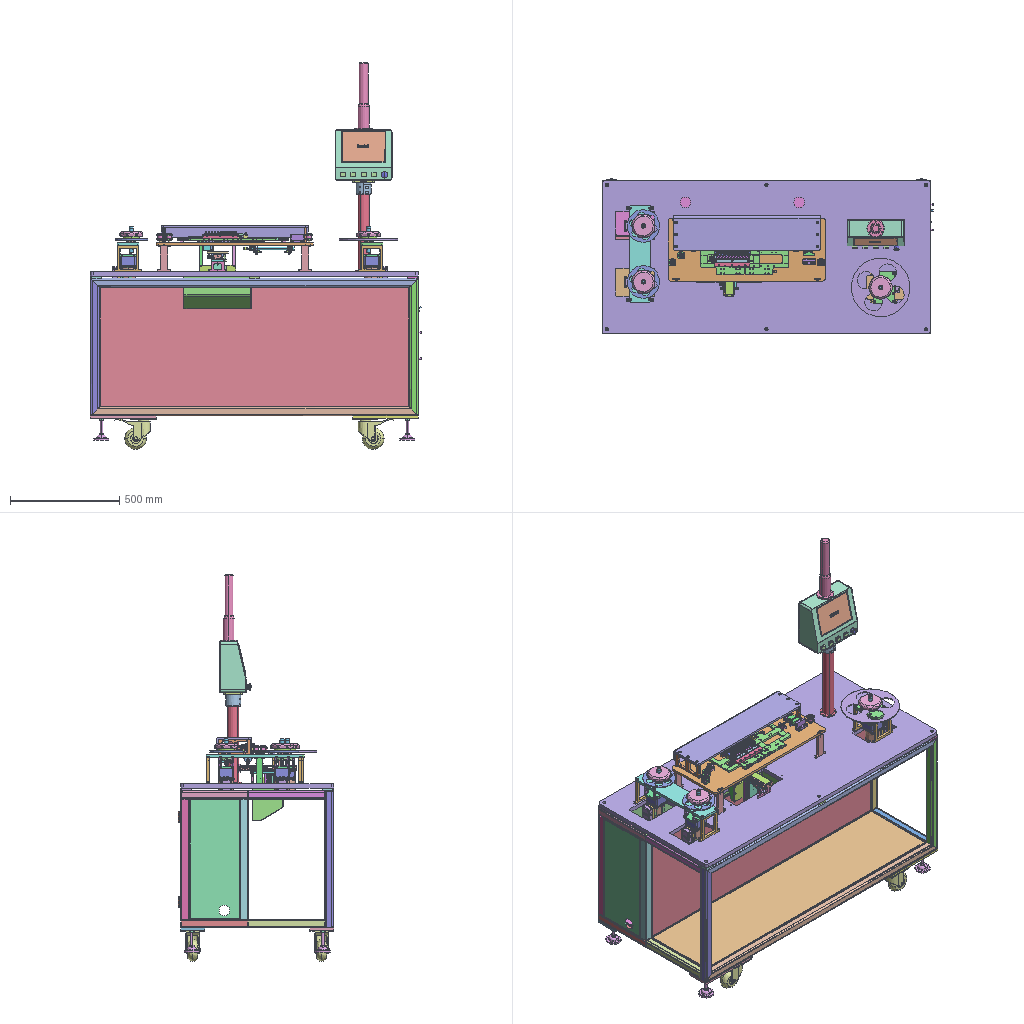Assembly | STEP file | 124 different items | 329 placed | box 1515 x 711 x 1768 mm
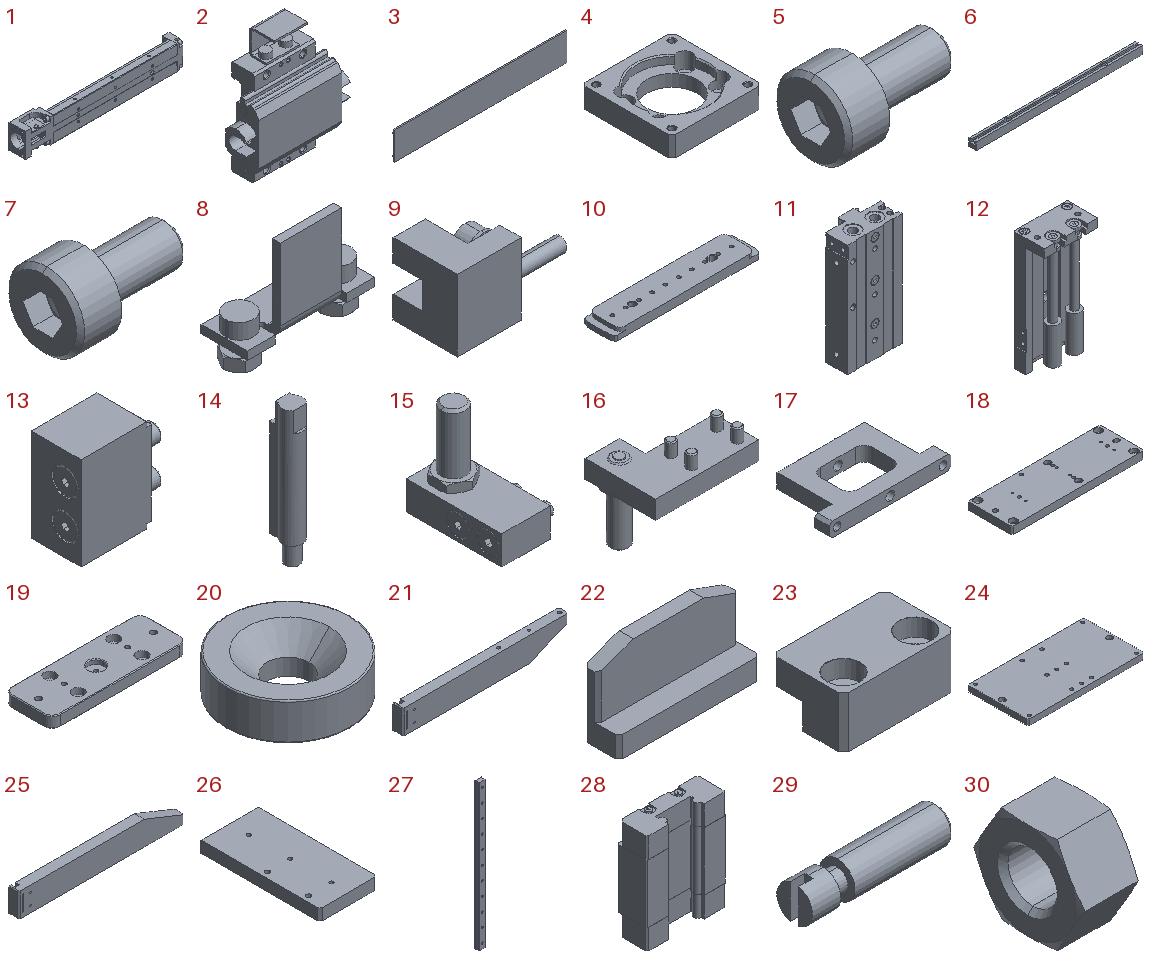Parts list (item | name | quantity | parent item | size | volume):
1 | QA-LX2005C_B1_A2038_200_EP3_b | x1 | in QA-LX2005C_B1_A2038_200_EP3 | 256 x 26.5 x 40 mm | 92553 mm3
2 | QA-LX2005C_B1_200_EP3_bl | x1 | in QA-LX2005C_B1_A2038_200_EP3 | 57 x 21 x 65.9 mm | 27894 mm3
3 | QA-LX2005C_B1_200_c | x1 | in QA-LX2005C_B1_A2038_200_EP3 | 216 x 3.2 x 35 mm | 15277 mm3
4 | QA-lx2001_A2038 | x1 | in QA-LX2005C_B1_A2038_200_EP3 | 38 x 38 x 8.5 mm | 7170 mm3
5 | QA-BOLT3_6 | x4 | in QA-LX2005C_B1_A2038_200_EP3 | 9 x 5.5 x 5.5 mm | 103.858 mm3
6 | QA-SENAT33H_208_V44_W104_X164_N3_5 | x1 | in QA-LX2005C_B1_A2038_200_EP3 | 208 x 9 x 9.5 mm | 12749 mm3
7 | QA-SCB3_6 | x3 | in QA-LX2005C_B1_A2038_200_EP3 | 9 x 5.5 x 5.5 mm | 103.858 mm3
8 | QA-PHOTO_SENSOR_br | x3 | in QA-LX2005C_B1_A2038_200_EP3 | 25.351 x 9 x 21 mm | 917.475 mm3
9 | QA-EE_SX91_R1M_lx | x3 | in QA-LX2005C_B1_A2038_200_EP3 | 21.25 x 12 x 14 mm | 1345 mm3
10 | QA-FB01 | x1 | in QA-FB0A | 150 x 32 x 9 mm | 39944 mm3
11 | QA-HI_MDX12x50-SD2BM2(0)_Bo | x1 | in QA-MDX12x50-SD2BM2 | 50 x 26.5 x 102 mm | 80346 mm3
12 | QA-HI_MDX12x50-SD2BM2(0)_Ro | x2 | in QA-MDX12x50-SD2BM2, QA-FB00 | 50 x 29 x 111 mm | 66088 mm3
13 | QA-HI_MDX-12 B | x1 | in QA-MDX12x50-SD2BM2 | 19.5 x 11 x 20.5 mm | 3566 mm3
14 | QA-HI_MDX-SD_2 | x2 | in QA-MDX12x50-SD2BM2 | 4 x 5.1 x 27.5 mm | 387.922 mm3
15 | QA-HI_MDX12_FB | x1 | in QA-MDX12x50-SD2BM2 | 20 x 31.5 x 33.5 mm | 6201 mm3
16 | QA-HI_MDX12_BB | x1 | in QA-MDX12x50-SD2BM2 | 45 x 31 x 38.5 mm | 10085 mm3
17 | QA-FB04 | x2 | in QA-FB00 | 84 x 48 x 10 mm | 20623 mm3
18 | QA-FB03 | x1 | in QA-FB00 | 180 x 60 x 10 mm | 103545 mm3
19 | QA-FB05 | x1 | in QA-FB00 | 96 x 34 x 8 mm | 24043 mm3
20 | QA-KZH10-3 | x1 | in QA-FB00 | 10 x 10 x 3 mm | 188.741 mm3
21 | QA-FB06 | x1 | in QA-FB00 | 206 x 12 x 30 mm | 66556 mm3
22 | QA-FB07 | x2 | in QA-FB00 | 20 x 5 x 11 mm | 541.763 mm3
23 | QA-FB08 | x2 | in QA-FB00 | 22 x 14 x 10 mm | 1976 mm3
24 | QA-FB09 | x1 | in QA-FB00 | 164 x 86 x 8 mm | 109937 mm3
25 | QA- Mirror FB06 | x1 | in QA-FB00 | 206 x 12 x 30 mm | 66556 mm3
26 | QA-FB10 | x1 | in QA-FB00 | 50 x 104 x 10 mm | 50937 mm3
27 | QA-r_SE2BL13_270 | x3 | in QA-SE2BL13_270, QA-SE2BL13_270-1, QA-0000-160616 | 12 x 7.5 x 270 mm | 21190 mm3
28 | QA-b_SEB13 | x6 | in QA-SE2BL13_270, QA-SE2BL13_270-1, QA-0000-160616 | 27 x 10 x 33.9 mm | 6982 mm3
29 | QA-BSPO5_20b | x11 | in QA-BSPO5_20, QA-BSPO5_20-1, QA-BSPO5_20-2, QA-BSPO5_20-3, QA-BSPO5_20-4, QA-BSPO5_20-5, QA-BSPO5_20-6, QA-BSPO5_20-7, QA-BSPO5_20-8, QA-BSPO5_20-9, QA-BSPO5_20-10 | 20 x 5 x 5 mm | 353.917 mm3
30 | QA-M5x0_8A | x22 | in QA-BSPO5_20, QA-BSPO5_25, QA-BSPO5_25-1, QA-BSPO5_25-2, QA-BSPO5_25-3, QA-BSPO5_25-4, QA-BSPO5_25-5, QA-BSPO5_25-6, QA-BSPO5_25-7, QA-BSPO5_25-8, QA-BSPO5_25-9, QA-BSPO5_25-10, QA-BSPO5_20-1, QA-BSPO5_20-2, QA-BSPO5_20-3, QA-BSPO5_20-4, QA-BSPO5_20-5, QA-BSPO5_20-6, QA-BSPO5_20-7, QA-BSPO5_20-8, QA-BSPO5_20-9, QA-BSPO5_20-10 | 4.7 x 9.238 x 8 mm | 194.282 mm3
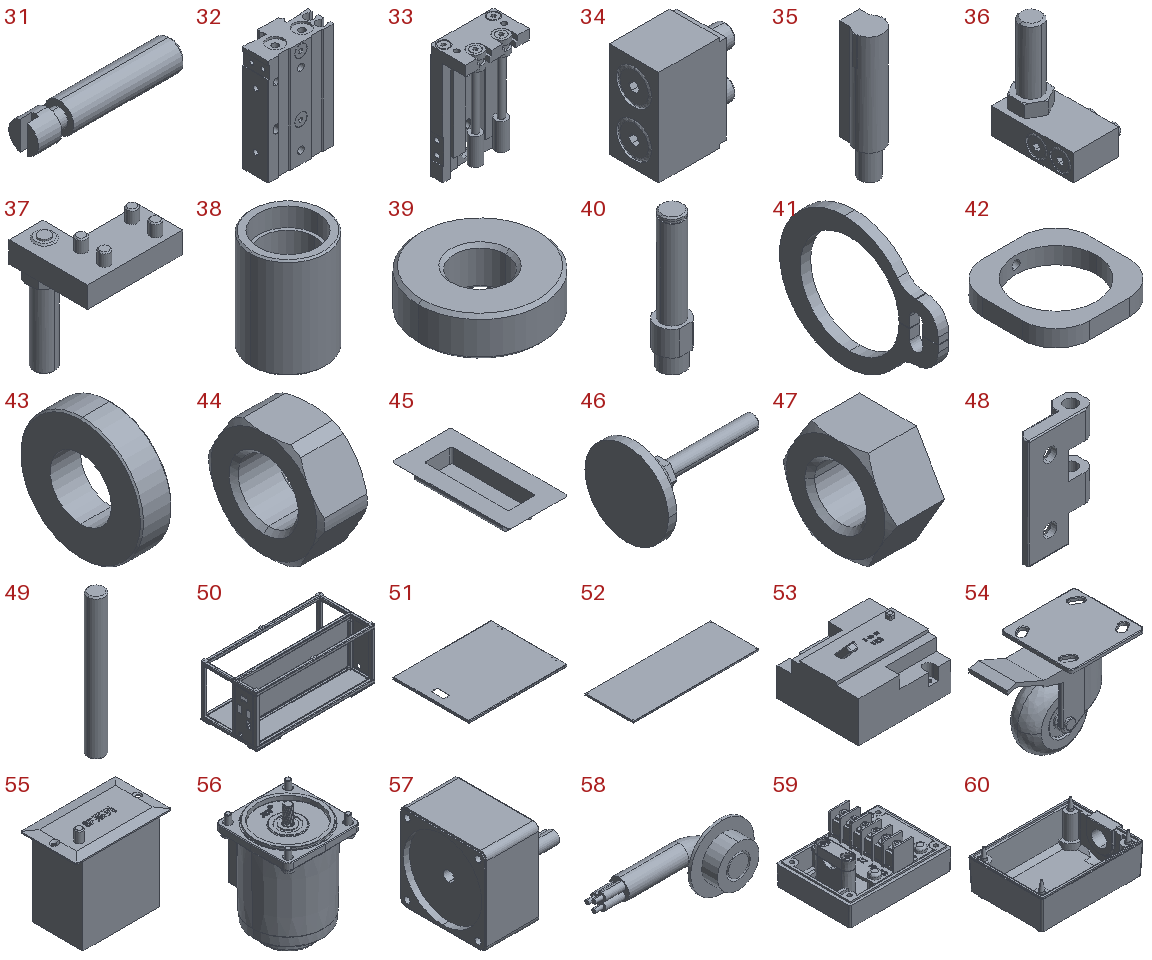31 | QA-BSPO5_25b | x11 | in QA-BSPO5_25, QA-BSPO5_25-1, QA-BSPO5_25-2, QA-BSPO5_25-3, QA-BSPO5_25-4, QA-BSPO5_25-5, QA-BSPO5_25-6, QA-BSPO5_25-7, QA-BSPO5_25-8, QA-BSPO5_25-9, QA-BSPO5_25-10 | 25 x 5 x 5 mm | 452.091 mm3
32 | QA-HI_MDX6x20-SG2BM2(0)_Bo | x1 | in QA-MDX6x20-SG2BM2 | 32 x 16 x 51.5 mm | 16782 mm3
33 | QA-HI_MDX6x20-SG2BM2(0)_Ro | x1 | in QA-MDX6x20-SG2BM2 | 32 x 18.5 x 57 mm | 12589 mm3
34 | QA-HI_MDX-6 B | x1 | in QA-MDX6x20-SG2BM2 | 13 x 7 x 13.5 mm | 935.094 mm3
35 | QA-HI_MDX-SG_2 | x2 | in QA-MDX6x20-SG2BM2 | 4 x 4.8 x 18 mm | 219.808 mm3
36 | QA-HI_MDX6_FB | x1 | in QA-MDX6x20-SG2BM2 | 13 x 19 x 26.37 mm | 1670 mm3
37 | QA-HI_MDX6_BB | x1 | in QA-MDX6x20-SG2BM2 | 22.5 x 18.7 x 29.3 mm | 2038 mm3
38 | QA-FC01 | x3 | in QA-FC00, QA-FC00-1, QA-FC00-2 | 24 x 24 x 32 mm | 6516 mm3
39 | QA-B698ZZ | x6 | in QA-FC00, QA-FC00-1, QA-FC00-2 | 19 x 19 x 6 mm | 1378 mm3
40 | QA-FC02 | x3 | in QA-FC00, QA-FC00-1, QA-FC00-2 | 11 x 10 x 49 mm | 2709 mm3
41 | QA-STWN8 | x3 | in QA-FC00, QA-FC00-1, QA-FC00-2 | 0.8 x 12.2 x 10 mm | 32.103 mm3
42 | QA-FC03 | x6 | in QA-FC00, QA-FC00-1, QA-FC00-2 | 32 x 32 x 5 mm | 2390 mm3
43 | QA-UWAUNS_washer-1 | x4 | in QA-UWAUNS-1, QA-UWAUNS-1-1 | 2 x 8 x 8 mm | 75.149 mm3
44 | QA-UWAUNS_nut-1 | x4 | in QA-UWAUNS-1, QA-UWAUNS-1-1 | 3.2 x 7.66 x 7 mm | 92.292 mm3
45 | QA-UWAUNS_1-1 | x2 | in QA-UWAUNS-1, QA-UWAUNS-1-1 | 60 x 120 x 15 mm | 28231 mm3
46 | QA-FJGN12_75pad-1 | x4 | in QA-FJGN12_75-1, QA-FJGN12_75-1-1, QA-FJGN12_75-1-2, QA-FJGN12_75-1-3 | 106 x 70 x 70 mm | 59651 mm3
47 | QA-FJGN12screw-1 | x4 | in QA-FJGN12_75-1, QA-FJGN12_75-1-1, QA-FJGN12_75-1-2, QA-FJGN12_75-1-3 | 10 x 21.939 x 19 mm | 2287 mm3
48 | QA-KHA50-1-1 | x8 | in QA-KHA50-1, 48, QA-KHA50-1-2, QA-KHA50-1-3 | 31 x 11.3 x 50 mm | 6837 mm3
49 | QA-KHA50-2-1 | x4 | in QA-KHA50-1, 48, QA-KHA50-1-2, QA-KHA50-1-3 | 6 x 6 x 50 mm | 1409 mm3
50 | QA-机箱-1(Default_As Machined_) | x1 | in QA-AD19 | 1500 x 700 x 650 mm | 12485783 mm3
51 | QA-Door panel B-1 | x2 | in QA-AD19 | 708 x 546 x 16.5 mm | 666860 mm3
52 | QA-衬Plate-1 | x1 | in QA-AD19 | 1416 x 546 x 18 mm | 1751680 mm3
53 | QA-N-33-HV-1 | x1 | in QA-AD19 | 90 x 80 x 56.121 mm | 279078 mm3
54 | QA-KVJHX100-1 | x4 | in QA-AD19 | 188.5 x 110 x 144.462 mm | 504709 mm3
55 | QA-SF系列调整器-1 | x3 | in QA-AD19 | 102 x 60 x 101 mm | 397007 mm3
56 | QA-15YT01-25-1 | x3 | in QA-15YT01-25, 56, 57 | 71.679 x 71.19 x 107.5 mm | 89869 mm3
57 | QA-15YT01-25-2 | x3 | in QA-15YT01-25, 56, 57 | 76 x 70.5 x 70.5 mm | 194650 mm3
58 | QA-15YT01-25-3 | x3 | in QA-15YT01-25, 56, 57 | 35 x 12.5 x 16 mm | 1115 mm3
59 | QA-15YT01-25-4 | x3 | in QA-15YT01-25, 56, 57 | 67 x 49 x 34.5 mm | 31444 mm3
60 | QA-15YT01-25-5 | x3 | in QA-15YT01-25, 56, 57 | 73.93 x 48.93 x 29.5 mm | 22748 mm3
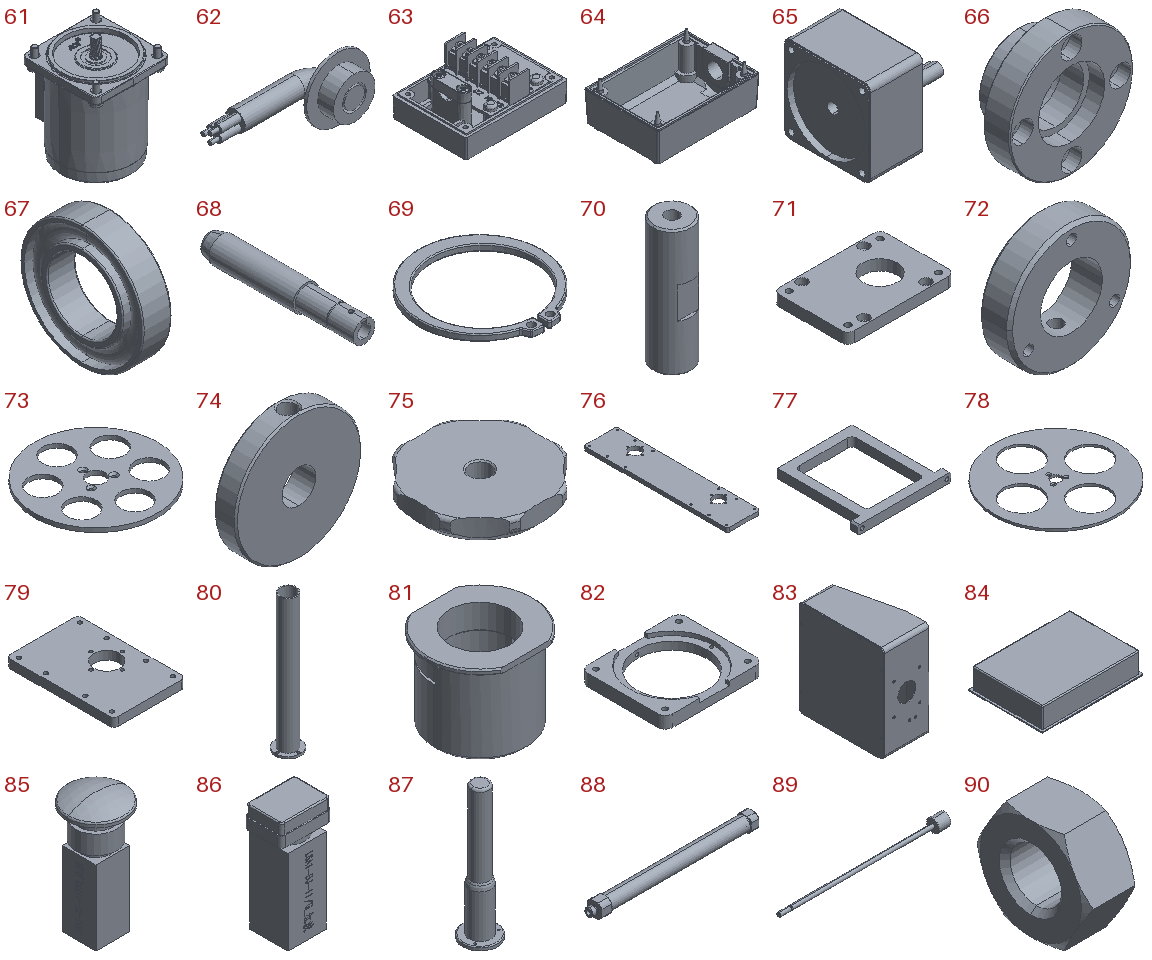61 | QA-70YS15G | x2 | in QA-06tp01-180, QA-06tp01-180-1 | 71.679 x 71.19 x 97.5 mm | 85810 mm3
62 | QA-YX_1 | x2 | in QA-06tp01-180, QA-06tp01-180-1 | 35 x 12.5 x 16 mm | 1115 mm3
63 | QA-JXH-X_1 | x2 | in QA-06tp01-180, QA-06tp01-180-1 | 67 x 49 x 34.5 mm | 31444 mm3
64 | QA-JXH-S_1 | x2 | in QA-06tp01-180, QA-06tp01-180-1 | 73.93 x 48.93 x 29.5 mm | 22748 mm3
65 | QA-70GK-H-180 | x2 | in QA-06tp01-180, QA-06tp01-180-1 | 76 x 70.5 x 70.5 mm | 194650 mm3
66 | QA-FC10 | x3 | in QA-Material discharge module, QA-放料模组-1, QA-Material receiving module | 56 x 24 x 56 mm | 24731 mm3
67 | QA-Bearing-B6903ZZ | x6 | in QA-Material discharge module, QA-放料模组-1, QA-Material receiving module | 7 x 30 x 30 mm | 2496 mm3
68 | QA-FC09 | x3 | in QA-Material discharge module, QA-放料模组-1, QA-Material receiving module | 20 x 120 x 19.5 mm | 30201 mm3
69 | QA-Retaining ring-KSTW17 | x3 | in QA-Material discharge module, QA-放料模组-1, QA-Material receiving module | 18.84 x 19.765 x 1 mm | 85.594 mm3
70 | QA-FC07 | x12 | in QA-Material discharge module, QA-放料模组-1, QA-Material receiving module | 12 x 12 x 40 mm | 4081 mm3
71 | QA-FC08 | x3 | in QA-Material discharge module, QA-放料模组-1, QA-Material receiving module | 100 x 70 x 10 mm | 57674 mm3
72 | QA-FC11 | x3 | in QA-Material discharge module, QA-放料模组-1, QA-Material receiving module | 40 x 10 x 40 mm | 8899 mm3
73 | QA-FC12 | x2 | in QA-Material discharge module, QA-放料模组-1 | 150 x 150 x 5 mm | 57214 mm3
74 | QA-FC15 | x3 | in QA-Material discharge module, QA-放料模组-1, QA-Material receiving module | 75 x 13 x 74.963 mm | 51433 mm3
75 | QA-FC13 | x3 | in QA-Material discharge module, QA-放料模组-1, QA-Material receiving module | 104.038 x 104.038 x 20 mm | 157045 mm3
76 | QA-FC04 | x1 | in QA-FC0A | 100 x 440 x 12 mm | 495046 mm3
77 | QA-FC06 | x4 | in QA-FC0A, QA-FC0B | 124 x 120 x 12 mm | 58795 mm3
78 | QA-FC14 | x1 | in QA-Material receiving module | 270 x 270 x 5 mm | 183467 mm3
79 | QA-FC05 | x1 | in QA-FC0B | 100 x 150 x 12 mm | 162249 mm3
80 | QA-TE01 | x1 | in QA-TE00 | 74 x 74 x 400 mm | 190414 mm3
81 | QA-TE02 | x1 | in QA-TE00 | 80 x 70 x 64 mm | 121771 mm3
82 | QA-TE03 | x1 | in QA-TE00 | 100 x 86 x 12 mm | 46511 mm3
83 | QA-TE04 | x1 | in QA-TE00 | 123 x 230 x 260 mm | 391275 mm3
84 | QA-MT6070IH | x1 | in QA-TE00 | 200 x 146 x 43 mm | 1146130 mm3
85 | QA-LSA1-BY-11TSB | x1 | in QA-TE00 | 30.8 x 30.8 x 65 mm | 21898 mm3
86 | QA-LSA1-BJ-11 | x4 | in QA-TE00 | 24 x 18 x 53 mm | 17646 mm3
87 | QA-TPWB4-L73ROG | x1 | in QA-TE00 | 80 x 80 x 307 mm | 491038 mm3
88 | QA-HI_SBA16x150-SB2-LB_B | x1 | in QA-SBA16x150-SB2-LB | 205 x 18 x 18 mm | 13813 mm3
89 | QA-HI_SBA16x150-LB_R | x1 | in QA-SBA16x150-SB2-LB | 210.5 x 16 x 16 mm | 6843 mm3
90 | QA-HI_N-M5x0.8_3 | x1 | in QA-SBA16x150-SB2-LB | 4 x 9.238 x 8 mm | 164.283 mm3
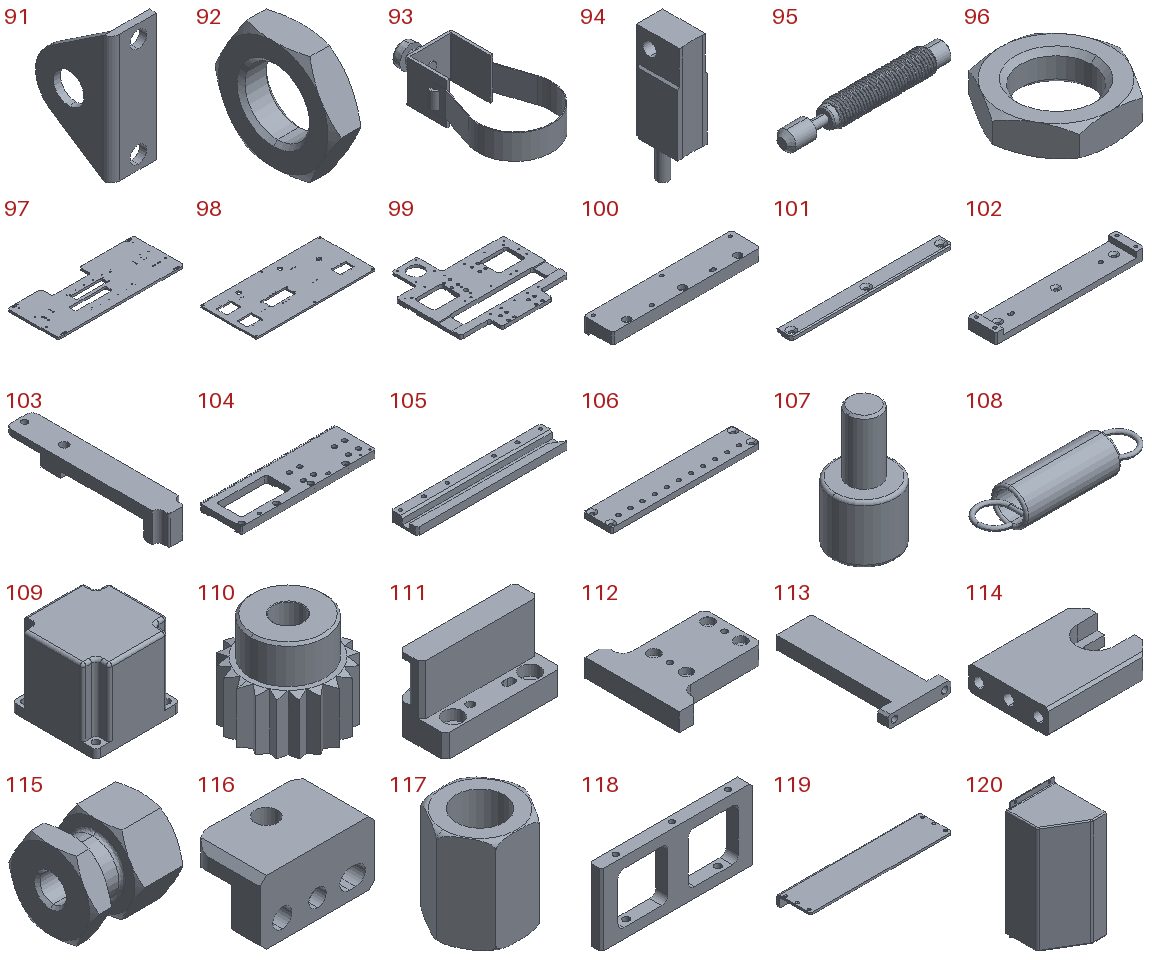91 | QA-HI_SBA-16-LB_(150) | x1 | in QA-SBA16x150-SB2-LB | 15 x 25 x 42 mm | 2467 mm3
92 | QA-HI_N-M10x1.0_3 | x1 | in QA-SBA16x150-SB2-LB | 4 x 17.321 x 15 mm | 513.744 mm3
93 | QA-HI_SBA16-SM_3 | x2 | in QA-SBA16x150-SB2-LB | 17.8 x 35.9 x 10 mm | 369.6 mm3
94 | QA-HI_SB-CS-130_3 | x2 | in QA-SBA16x150-SB2-LB | 8 x 11.8 x 36 mm | 2270 mm3
95 | QA-SKSC0806-1 | x2 | in QA-SKSC0806, 95 | 55.353 x 8 x 8 mm | 1947 mm3
96 | QA-SKSC0806-2 | x4 | in QA-SKSC0806, 95 | 12.702 x 11 x 3 mm | 190.264 mm3
97 | QA-AD01 | x1 | in QA-0000-160616 | 720 x 288 x 12 mm | 2124409 mm3
98 | QA-AD02 | x1 | in QA-0000-160616 | 1500 x 700 x 20 mm | 18757856 mm3
99 | QA-AD03 | x2 | in QA-0000-160616 | 270 x 258 x 10 mm | 320540 mm3
100 | QA-AD04 | x1 | in QA-0000-160616 | 160 x 32 x 15.1 mm | 62990 mm3
101 | QA-AD05 | x1 | in QA-0000-160616 | 160 x 16 x 4 mm | 9462 mm3
102 | QA-AD06 | x1 | in QA-0000-160616 | 166.5 x 32 x 12 mm | 34292 mm3
103 | QA-AD07 | x11 | in QA-0000-160616 | 13.5 x 80 x 14.8 mm | 6677 mm3
104 | QA-AD08 | x1 | in QA-0000-160616 | 195 x 60 x 10 mm | 78945 mm3
105 | QA-AD09 | x1 | in QA-0000-160616 | 160 x 28 x 10.5 mm | 32238 mm3
106 | QA-AD10 | x1 | in QA-0000-160616 | 166.5 x 32 x 6 mm | 30437 mm3
107 | QA-CFM3-6 | x11 | in QA-0000-160616 | 6 x 6 x 11.5 mm | 192.07 mm3
108 | QA-AWU6_25 | x11 | in QA-0000-160616 | 26.4 x 6 x 6 mm | 193.836 mm3
109 | QA-SM57-51C | x1 | in QA-0000-160616 | 56.4 x 56.4 x 73.2 mm | 150583 mm3
110 | QA-GER1.0-20-W12-B-H6.35 | x1 | in QA-0000-160616 | 22 x 22 x 20 mm | 4666 mm3
111 | QA-AD11 | x1 | in QA-0000-160616 | 60 x 24 x 38 mm | 30322 mm3
112 | QA-AD12 | x1 | in QA-0000-160616 | 56 x 52 x 10 mm | 19264 mm3
113 | QA-AD13 | x4 | in QA-0000-160616 | 60 x 120 x 12 mm | 50441 mm3
114 | QA-AD14 | x1 | in QA-0000-160616 | 43 x 32 x 10 mm | 11347 mm3
115 | QA-KFJR5-0.8-4 | x1 | in QA-0000-160616 | 14 x 13.856 x 12 mm | 1253 mm3
116 | QA-AD15 | x2 | in QA-0000-160616 | 36 x 22 x 20 mm | 8518 mm3
117 | QA-SKST801 | x2 | in QA-0000-160616 | 12.702 x 11 x 14 mm | 925.966 mm3
118 | QA-AD17 | x2 | in QA-0000-160616 | 150 x 12 x 70 mm | 65829 mm3
119 | QA-AD16 | x1 | in QA-0000-160616 | 672 x 160 x 55 mm | 1359289 mm3
120 | QA-AD18 | x1 | in QA-0000-160616 | 140 x 150 x 342 mm | 227668 mm3
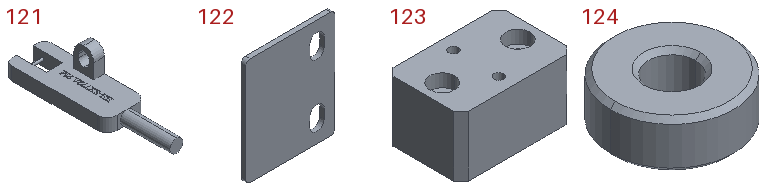121 | QA-EE-SX772A 2M | x1 | in QA-0000-160616 | 12 x 46 x 19.1 mm | 1673 mm3
122 | QA-AD20 | x1 | in QA-0000-160616 | 20 x 1 x 24 mm | 450.257 mm3
123 | QA-AD21 | x1 | in QA-0000-160616 | 30 x 20 x 16 mm | 8932 mm3
124 | QA-KGHA5-13 | x3 | in QA-0000-160616 | 13 x 13 x 5 mm | 551.35 mm3
Placements (level | parent | child | x y z in mm | rotation matrix by rows), first 242 of 386 lines:
1 | QA-0000-160616 | QA-FB00 | -62.867 62.015 497.223 | 1 0 0 0 0 -1 0 1 0
2 | QA-FB00 | QA-LX2005C_B1_A2038_200_EP3 | -1.553 34.777 194.0 | 0 0 -1 0 1 0 1 0 0
3 | QA-LX2005C_B1_A2038_200_EP3 | QA-LX2005C_B1_A2038_200_EP3_b | -128.0 -0.0 -0.0 | 1 0 0 0 1 0 0 0 1
3 | QA-LX2005C_B1_A2038_200_EP3 | QA-LX2005C_B1_200_EP3_bl | -42.0 -0.0 -0.0 | 1 0 0 0 1 0 0 0 1
3 | QA-LX2005C_B1_A2038_200_EP3 | QA-LX2005C_B1_200_c | -128.0 -0.0 -0.0 | 1 0 0 0 1 0 0 0 1
3 | QA-LX2005C_B1_A2038_200_EP3 | QA-lx2001_A2038 | -132.25 13.0 -0.0 | 0 0 -1 0 1 0 1 0 0
3 | QA-LX2005C_B1_A2038_200_EP3 | QA-BOLT3_6 | -129.8 5.75 -12.557 | 1 0 0 0 -1 0 0 0 -1
3 | QA-LX2005C_B1_A2038_200_EP3 | QA-BOLT3_6 | -129.8 20.25 12.557 | 1 0 0 0 -1 0 0 0 -1
3 | QA-LX2005C_B1_A2038_200_EP3 | QA-BOLT3_6 | -129.8 20.25 -12.557 | 1 0 0 0 -1 0 0 0 -1
3 | QA-LX2005C_B1_A2038_200_EP3 | QA-BOLT3_6 | -129.8 5.75 12.557 | 1 0 0 0 -1 0 0 0 -1
3 | QA-LX2005C_B1_A2038_200_EP3 | QA-SENAT33H_208_V44_W104_X164_N3_5 | -86.0 5.5 20.0 | 1 0 0 0 1 0 0 0 1
3 | QA-LX2005C_B1_A2038_200_EP3 | QA-SCB3_6 | 78.0 5.5 22.0 | 0 0 -1 0 -1 0 -1 0 0
3 | QA-LX2005C_B1_A2038_200_EP3 | QA-SCB3_6 | -42.0 5.5 22.0 | 0 0 -1 0 -1 0 -1 0 0
3 | QA-LX2005C_B1_A2038_200_EP3 | QA-SCB3_6 | 18.0 5.5 22.0 | 0 0 -1 0 -1 0 -1 0 0
3 | QA-LX2005C_B1_A2038_200_EP3 | QA-PHOTO_SENSOR_br | -38.0 1.0 29.5 | 1 0 0 0 1 0 0 0 1
3 | QA-LX2005C_B1_A2038_200_EP3 | QA-PHOTO_SENSOR_br | 74.0 1.0 29.5 | 1 0 0 0 1 0 0 0 1
3 | QA-LX2005C_B1_A2038_200_EP3 | QA-PHOTO_SENSOR_br | 18.0 1.0 29.5 | 1 0 0 0 1 0 0 0 1
3 | QA-LX2005C_B1_A2038_200_EP3 | QA-EE_SX91_R1M_lx | 74.0 2.6 46.1 | -1 0 0 0 1 0 0 0 -1
3 | QA-LX2005C_B1_A2038_200_EP3 | QA-EE_SX91_R1M_lx | -38.0 2.6 46.1 | -1 0 0 0 1 0 0 0 -1
3 | QA-LX2005C_B1_A2038_200_EP3 | QA-EE_SX91_R1M_lx | 18.0 2.6 46.1 | -1 0 0 0 1 0 0 0 -1
2 | QA-FB00 | QA-FB0A | 1.597 -18.223 137.473 | 1 0 0 0 0 1 0 -1 0
3 | QA-FB0A | QA-FB01 | -3.15 -14.527 136.0 | 1 0 0 0 1 0 0 0 1
2 | QA-FB00 | QA-MDX12x50-SD2BM2 | -1.553 -79.223 207.0 | -1 0 0 0 0 -1 0 -1 0
3 | QA-MDX12x50-SD2BM2 | QA-HI_MDX12x50-SD2BM2(0)_Bo | -0.0 -0.0 -0.0 | 1 0 0 0 1 0 0 0 1
3 | QA-MDX12x50-SD2BM2 | QA-HI_MDX12x50-SD2BM2(0)_Ro | -0.0 -0.0 -0.0 | 1 0 0 0 1 0 0 0 1
3 | QA-MDX12x50-SD2BM2 | QA-HI_MDX-12 B | -25.0 24.0 -73.75 | 1 0 0 0 1 0 0 0 1
3 | QA-MDX12x50-SD2BM2 | QA-HI_MDX-SD_2 | 20.0 6.0 -102.0 | 0 1 0 1 0 0 0 0 -1
3 | QA-MDX12x50-SD2BM2 | QA-HI_MDX-SD_2 | 20.0 14.0 -0.0 | 0 1 0 -1 0 0 0 0 1
3 | QA-MDX12x50-SD2BM2 | QA-HI_MDX12_FB | -25.0 5.0 -6.75 | 1 0 0 0 1 0 0 0 1
3 | QA-MDX12x50-SD2BM2 | QA-HI_MDX12_BB | -0.0 5.0 -102.0 | 1 0 0 0 1 0 0 0 1
2 | QA-FB00 | QA-FB04 | -1.553 0.7766 115.0 | 1 0 0 0 1 0 0 0 1
2 | QA-FB00 | QA-FB04 | -1.553 0.7766 279.0 | 1 0 0 0 1 0 0 0 1
2 | QA-FB00 | QA-FB03 | -1.553 24.777 202.0 | 0 1 0 0 0 1 1 0 0
2 | QA-FB00 | QA-FB05 | -1.553 61.777 152.0 | 1 0 0 0 0 1 0 -1 0
2 | QA-FB00 | QA-KZH10-3 | -1.553 66.577 152.0 | 1 0 0 0 0 1 0 -1 0
2 | QA-FB00 | QA-FB06 | -83.553 125.877 137.0 | 0 1 0 -1 0 0 0 0 1
2 | QA-FB00 | QA-FB07 | 84.447 121.277 152.0 | 0 0 -1 0 1 0 1 0 -0
2 | QA-FB00 | QA-FB07 | -87.553 121.277 152.0 | 0 0 1 0 1 0 -1 0 -0
2 | QA-FB00 | QA-FB08 | 80.447 107.277 152.0 | 0 0 1 0 1 0 -1 0 0
2 | QA-FB00 | QA-FB08 | -83.553 107.277 152.0 | 0 0 -1 0 1 0 1 0 0
2 | QA-FB00 | QA-FB09 | -1.553 -37.123 167.0 | 1 0 0 0 1 0 0 0 1
2 | QA-FB00 | QA- Mirror FB06 | 80.447 125.877 137.0 | 0 -1 0 -1 0 0 0 0 -1
2 | QA-FB00 | QA-FB10 | -1.553 -27.223 217.0 | -1 0 0 0 1 0 0 0 -1
2 | QA-FB00 | QA-HI_MDX12x50-SD2BM2(0)_Ro | -1.553 -129.223 207.0 | -1 0 0 0 0 -1 0 -1 0
1 | QA-0000-160616 | QA-SE2BL13_270 | 148.58 -3.985 606.0 | 0 0 -1 -1 0 0 0 1 0
2 | QA-SE2BL13_270 | QA-r_SE2BL13_270 | -0.0 -0.0 -0.0 | 1 0 0 0 1 0 0 0 1
2 | QA-SE2BL13_270 | QA-b_SEB13 | -0.0 3.0 174.889 | 1 0 0 0 1 0 0 0 1
2 | QA-SE2BL13_270 | QA-b_SEB13 | -0.0 3.0 244.889 | 1 0 0 0 1 0 0 0 1
1 | QA-0000-160616 | QA-SE2BL13_270-1 | 148.58 -145.985 606.0 | 0 0 -1 -1 0 0 0 1 0
2 | QA-SE2BL13_270-1 | QA-r_SE2BL13_270 | -0.0 -0.0 -0.0 | 1 0 0 0 1 0 0 0 1
2 | QA-SE2BL13_270-1 | QA-b_SEB13 | -0.0 3.0 244.889 | 1 0 0 0 1 0 0 0 1
2 | QA-SE2BL13_270-1 | QA-b_SEB13 | -0.0 3.0 174.889 | 1 0 0 0 1 0 0 0 1
1 | QA-0000-160616 | QA-BSPO5_20 | -117.77 -65.985 660.0 | 0 -0.866 0.5 0 0.5 0.866 -1 0 -0
2 | QA-BSPO5_20 | QA-BSPO5_20b | -0.0 -0.0 -0.0 | 1 0 0 0 1 0 0 0 1
2 | QA-BSPO5_20 | QA-M5x0_8A | 12.65 0.0 -0.0 | -1 0 0 0 -1 0 0 0 1
1 | QA-0000-160616 | QA-BSPO5_25 | -118.42 -28.985 657.9 | 0 0 1 0 1 0 -1 0 0
2 | QA-BSPO5_25 | QA-M5x0_8A | 16.65 -0.0 -0.0 | -1 0 0 0 -1 0 0 0 1
2 | QA-BSPO5_25 | QA-BSPO5_25b | -0.0 -0.0 -0.0 | 1 0 0 0 1 0 0 0 1
1 | QA-0000-160616 | QA-BSPO5_25-1 | -104.92 -28.985 657.9 | 0 0 1 0 1 0 -1 0 0
2 | QA-BSPO5_25-1 | QA-M5x0_8A | 16.65 -0.0 -0.0 | -1 0 0 0 -1 0 0 0 1
2 | QA-BSPO5_25-1 | QA-BSPO5_25b | -0.0 -0.0 -0.0 | 1 0 0 0 1 0 0 0 1
1 | QA-0000-160616 | QA-BSPO5_25-2 | -91.42 -28.985 657.9 | 0 0 1 0 1 0 -1 0 0
2 | QA-BSPO5_25-2 | QA-M5x0_8A | 16.65 -0.0 -0.0 | -1 0 0 0 -1 0 0 0 1
2 | QA-BSPO5_25-2 | QA-BSPO5_25b | -0.0 -0.0 -0.0 | 1 0 0 0 1 0 0 0 1
1 | QA-0000-160616 | QA-BSPO5_25-3 | -77.92 -28.985 657.9 | 0 0 1 0 1 0 -1 0 0
2 | QA-BSPO5_25-3 | QA-M5x0_8A | 16.65 -0.0 -0.0 | -1 0 0 0 -1 0 0 0 1
2 | QA-BSPO5_25-3 | QA-BSPO5_25b | -0.0 -0.0 -0.0 | 1 0 0 0 1 0 0 0 1
1 | QA-0000-160616 | QA-BSPO5_25-4 | -64.42 -28.985 657.9 | 0 0 1 0 1 0 -1 0 0
2 | QA-BSPO5_25-4 | QA-M5x0_8A | 16.65 -0.0 -0.0 | -1 0 0 0 -1 0 0 0 1
2 | QA-BSPO5_25-4 | QA-BSPO5_25b | -0.0 -0.0 -0.0 | 1 0 0 0 1 0 0 0 1
1 | QA-0000-160616 | QA-BSPO5_25-5 | -50.92 -28.985 657.9 | 0 0 1 0 1 0 -1 0 0
2 | QA-BSPO5_25-5 | QA-M5x0_8A | 16.65 -0.0 -0.0 | -1 0 0 0 -1 0 0 0 1
2 | QA-BSPO5_25-5 | QA-BSPO5_25b | -0.0 -0.0 -0.0 | 1 0 0 0 1 0 0 0 1
1 | QA-0000-160616 | QA-BSPO5_25-6 | -37.42 -28.985 657.9 | 0 0 1 0 1 0 -1 0 0
2 | QA-BSPO5_25-6 | QA-M5x0_8A | 16.65 -0.0 -0.0 | -1 0 0 0 -1 0 0 0 1
2 | QA-BSPO5_25-6 | QA-BSPO5_25b | -0.0 -0.0 -0.0 | 1 0 0 0 1 0 0 0 1
1 | QA-0000-160616 | QA-BSPO5_25-7 | -23.92 -28.985 657.9 | 0 0 1 0 1 0 -1 0 0
2 | QA-BSPO5_25-7 | QA-M5x0_8A | 16.65 -0.0 -0.0 | -1 0 0 0 -1 0 0 0 1
2 | QA-BSPO5_25-7 | QA-BSPO5_25b | -0.0 -0.0 -0.0 | 1 0 0 0 1 0 0 0 1
1 | QA-0000-160616 | QA-BSPO5_25-8 | -10.42 -28.985 657.9 | 0 0 1 0 1 0 -1 0 0
2 | QA-BSPO5_25-8 | QA-M5x0_8A | 16.65 -0.0 -0.0 | -1 0 0 0 -1 0 0 0 1
2 | QA-BSPO5_25-8 | QA-BSPO5_25b | -0.0 -0.0 -0.0 | 1 0 0 0 1 0 0 0 1
1 | QA-0000-160616 | QA-BSPO5_25-9 | 3.08 -28.985 657.9 | 0 0 1 0 1 0 -1 0 0
2 | QA-BSPO5_25-9 | QA-M5x0_8A | 16.65 -0.0 -0.0 | -1 0 0 0 -1 0 0 0 1
2 | QA-BSPO5_25-9 | QA-BSPO5_25b | -0.0 -0.0 -0.0 | 1 0 0 0 1 0 0 0 1
1 | QA-0000-160616 | QA-BSPO5_25-10 | 16.58 -28.985 657.9 | 0 0 1 0 1 0 -1 0 0
2 | QA-BSPO5_25-10 | QA-M5x0_8A | 16.65 -0.0 -0.0 | -1 0 0 0 -1 0 0 0 1
2 | QA-BSPO5_25-10 | QA-BSPO5_25b | -0.0 -0.0 -0.0 | 1 0 0 0 1 0 0 0 1
1 | QA-0000-160616 | QA-BSPO5_20-1 | -104.27 -65.985 660.0 | 0 -0.866 0.5 0 0.5 0.866 -1 0 -0
2 | QA-BSPO5_20-1 | QA-BSPO5_20b | -0.0 -0.0 -0.0 | 1 0 0 0 1 0 0 0 1
2 | QA-BSPO5_20-1 | QA-M5x0_8A | 12.65 0.0 -0.0 | -1 0 0 0 -1 0 0 0 1
1 | QA-0000-160616 | QA-BSPO5_20-2 | -90.77 -65.985 660.0 | 0 -0.866 0.5 0 0.5 0.866 -1 0 -0
2 | QA-BSPO5_20-2 | QA-BSPO5_20b | -0.0 -0.0 -0.0 | 1 0 0 0 1 0 0 0 1
2 | QA-BSPO5_20-2 | QA-M5x0_8A | 12.65 0.0 -0.0 | -1 0 0 0 -1 0 0 0 1
1 | QA-0000-160616 | QA-BSPO5_20-3 | -77.27 -65.985 660.0 | 0 -0.866 0.5 0 0.5 0.866 -1 0 -0
2 | QA-BSPO5_20-3 | QA-BSPO5_20b | -0.0 -0.0 -0.0 | 1 0 0 0 1 0 0 0 1
2 | QA-BSPO5_20-3 | QA-M5x0_8A | 12.65 0.0 -0.0 | -1 0 0 0 -1 0 0 0 1
1 | QA-0000-160616 | QA-BSPO5_20-4 | -63.77 -65.985 660.0 | 0 -0.866 0.5 0 0.5 0.866 -1 0 -0
2 | QA-BSPO5_20-4 | QA-BSPO5_20b | -0.0 -0.0 -0.0 | 1 0 0 0 1 0 0 0 1
2 | QA-BSPO5_20-4 | QA-M5x0_8A | 12.65 0.0 -0.0 | -1 0 0 0 -1 0 0 0 1
1 | QA-0000-160616 | QA-BSPO5_20-5 | -50.27 -65.985 660.0 | 0 -0.866 0.5 0 0.5 0.866 -1 0 -0
2 | QA-BSPO5_20-5 | QA-BSPO5_20b | -0.0 -0.0 -0.0 | 1 0 0 0 1 0 0 0 1
2 | QA-BSPO5_20-5 | QA-M5x0_8A | 12.65 0.0 -0.0 | -1 0 0 0 -1 0 0 0 1
1 | QA-0000-160616 | QA-BSPO5_20-6 | -36.77 -65.985 660.0 | 0 -0.866 0.5 0 0.5 0.866 -1 0 -0
2 | QA-BSPO5_20-6 | QA-BSPO5_20b | -0.0 -0.0 -0.0 | 1 0 0 0 1 0 0 0 1
2 | QA-BSPO5_20-6 | QA-M5x0_8A | 12.65 0.0 -0.0 | -1 0 0 0 -1 0 0 0 1
1 | QA-0000-160616 | QA-BSPO5_20-7 | -23.27 -65.985 660.0 | 0 -0.866 0.5 0 0.5 0.866 -1 0 -0
2 | QA-BSPO5_20-7 | QA-BSPO5_20b | -0.0 -0.0 -0.0 | 1 0 0 0 1 0 0 0 1
2 | QA-BSPO5_20-7 | QA-M5x0_8A | 12.65 0.0 -0.0 | -1 0 0 0 -1 0 0 0 1
1 | QA-0000-160616 | QA-BSPO5_20-8 | -9.77 -65.985 660.0 | 0 -0.866 0.5 0 0.5 0.866 -1 0 -0
2 | QA-BSPO5_20-8 | QA-BSPO5_20b | -0.0 -0.0 -0.0 | 1 0 0 0 1 0 0 0 1
2 | QA-BSPO5_20-8 | QA-M5x0_8A | 12.65 0.0 -0.0 | -1 0 0 0 -1 0 0 0 1
1 | QA-0000-160616 | QA-BSPO5_20-9 | 3.73 -65.985 660.0 | 0 -0.866 0.5 0 0.5 0.866 -1 0 -0
2 | QA-BSPO5_20-9 | QA-BSPO5_20b | -0.0 -0.0 -0.0 | 1 0 0 0 1 0 0 0 1
2 | QA-BSPO5_20-9 | QA-M5x0_8A | 12.65 0.0 -0.0 | -1 0 0 0 -1 0 0 0 1
1 | QA-0000-160616 | QA-BSPO5_20-10 | 17.23 -65.985 660.0 | 0 -0.866 0.5 0 0.5 0.866 -1 0 -0
2 | QA-BSPO5_20-10 | QA-BSPO5_20b | -0.0 -0.0 -0.0 | 1 0 0 0 1 0 0 0 1
2 | QA-BSPO5_20-10 | QA-M5x0_8A | 12.65 0.0 -0.0 | -1 0 0 0 -1 0 0 0 1
1 | QA-0000-160616 | QA-MDX6x20-SG2BM2 | 299.58 -58.485 606.0 | 1 0 0 0 0 -1 0 1 0
2 | QA-MDX6x20-SG2BM2 | QA-HI_MDX6x20-SG2BM2(0)_Bo | -0.0 -0.0 -0.0 | 1 0 0 0 1 0 0 0 1
2 | QA-MDX6x20-SG2BM2 | QA-HI_MDX6x20-SG2BM2(0)_Ro | -0.0 -0.0 -0.0 | 1 0 0 0 1 0 0 0 1
2 | QA-MDX6x20-SG2BM2 | QA-HI_MDX-6 B | -16.0 16.5 -37.25 | 1 0 0 0 1 0 0 0 1
2 | QA-MDX6x20-SG2BM2 | QA-HI_MDX-SG_2 | 13.0 9.0 -0.0 | 0 1 0 -1 0 0 0 0 1
2 | QA-MDX6x20-SG2BM2 | QA-HI_MDX-SG_2 | 13.0 3.3 -51.5 | 0 1 0 1 0 0 0 0 -1
2 | QA-MDX6x20-SG2BM2 | QA-HI_MDX6_FB | -16.0 3.0 -5.0 | 1 0 0 0 1 0 0 0 1
2 | QA-MDX6x20-SG2BM2 | QA-HI_MDX6_BB | -0.0 3.0 -51.5 | 1 0 0 0 1 0 0 0 1
1 | QA-0000-160616 | QA-FC00 | -329.456 -103.569 589.0 | 0.8983 0.4394 0 -0.4394 0.8983 0 0 0 1
2 | QA-FC00 | QA-FC01 | 3.349 0.062 26.0 | 1 0 0 0 1 0 0 0 1
2 | QA-FC00 | QA-B698ZZ | 3.349 0.062 26.0 | 1 0 0 0 1 0 0 0 1
2 | QA-FC00 | QA-B698ZZ | 3.349 0.062 52.0 | 1 0 0 0 1 0 0 0 1
2 | QA-FC00 | QA-FC02 | 3.349 0.062 26.0 | 0.8983 -0.4394 0 0.4394 0.8983 0 0 0 1
2 | QA-FC00 | QA-STWN8 | 3.349 0.062 58.4 | 0 0 -1 0 1 0 1 0 0
2 | QA-FC00 | QA-FC03 | 3.349 0.062 50.0 | 0.8983 -0.4394 0 0.4394 0.8983 0 0 0 1
2 | QA-FC00 | QA-FC03 | 3.349 0.062 31.0 | 0.8983 -0.4394 0 0.4394 0.8983 0 0 0 1
1 | QA-0000-160616 | QA-FC00-1 | -289.456 -71.569 589.0 | 0.8983 0.4394 0 -0.4394 0.8983 0 0 0 1
2 | QA-FC00-1 | QA-FC01 | 3.349 0.062 26.0 | 1 0 0 0 1 0 0 0 1
2 | QA-FC00-1 | QA-B698ZZ | 3.349 0.062 52.0 | 1 0 0 0 1 0 0 0 1
2 | QA-FC00-1 | QA-B698ZZ | 3.349 0.062 26.0 | 1 0 0 0 1 0 0 0 1
2 | QA-FC00-1 | QA-FC02 | 3.349 0.062 26.0 | 0.8983 -0.4394 0 0.4394 0.8983 0 0 0 1
2 | QA-FC00-1 | QA-STWN8 | 3.349 0.062 58.4 | 0 0 -1 0 1 0 1 0 0
2 | QA-FC00-1 | QA-FC03 | 3.349 0.062 50.0 | 0.8983 -0.4394 0 0.4394 0.8983 0 0 0 1
2 | QA-FC00-1 | QA-FC03 | 3.349 0.062 31.0 | 0.8983 -0.4394 0 0.4394 0.8983 0 0 0 1
1 | QA-0000-160616 | QA-FC00-2 | 350.544 -103.569 589.0 | 0.8983 0.4394 0 -0.4394 0.8983 0 0 0 1
2 | QA-FC00-2 | QA-FC01 | 3.349 0.062 26.0 | 1 0 0 0 1 0 0 0 1
2 | QA-FC00-2 | QA-B698ZZ | 3.349 0.062 26.0 | 1 0 0 0 1 0 0 0 1
2 | QA-FC00-2 | QA-B698ZZ | 3.349 0.062 52.0 | 1 0 0 0 1 0 0 0 1
2 | QA-FC00-2 | QA-FC02 | 3.349 0.062 26.0 | 0.8983 -0.4394 0 0.4394 0.8983 0 0 0 1
2 | QA-FC00-2 | QA-STWN8 | 3.349 0.062 58.4 | 0 0 -1 0 1 0 1 0 0
2 | QA-FC00-2 | QA-FC03 | 3.349 0.062 50.0 | 0.8983 -0.4394 0 0.4394 0.8983 0 0 0 1
2 | QA-FC00-2 | QA-FC03 | 3.349 0.062 31.0 | 0.8983 -0.4394 0 0.4394 0.8983 0 0 0 1
1 | QA-0000-160616 | QA-AD19 | -89.579 192.173 -986.0 | -1 0 0 0 -1 0 0 0 1
2 | QA-AD19 | QA-UWAUNS-1 | -123.158 -77.842 1112.0 | 1 0 0 0 0 -1 0 1 -0
3 | QA-UWAUNS-1 | QA-UWAUNS_washer-1 | -0.0 -50.0 -2.0 | 0 0 -1 0 -1 0 -1 0 -0
3 | QA-UWAUNS-1 | QA-UWAUNS_washer-1 | -0.0 50.0 -2.0 | 0 0 -1 0 -1 0 -1 0 -0
3 | QA-UWAUNS-1 | QA-UWAUNS_nut-1 | -0.0 -50.0 -4.0 | 0 0 -1 0 -1 0 -1 0 -0
3 | QA-UWAUNS-1 | QA-UWAUNS_nut-1 | 0.0 50.0 -4.0 | 0 0 -1 0 -1 0 -1 0 -0
3 | QA-UWAUNS-1 | QA-UWAUNS_1-1 | -0.0 -0.0 -0.0 | 1 0 0 0 1 0 0 0 1
2 | QA-AD19 | QA-UWAUNS-1-1 | -263.158 -77.842 1112.0 | -1 0 0 0 0 -1 0 -1 0
3 | QA-UWAUNS-1-1 | QA-UWAUNS_washer-1 | -0.0 -50.0 -2.0 | 0 0 -1 0 -1 0 -1 0 0
3 | QA-UWAUNS-1-1 | QA-UWAUNS_washer-1 | -0.0 50.0 -2.0 | 0 0 -1 0 -1 0 -1 0 0
3 | QA-UWAUNS-1-1 | QA-UWAUNS_nut-1 | -0.0 50.0 -4.0 | 0 0 -1 0 -1 0 -1 0 0
3 | QA-UWAUNS-1-1 | QA-UWAUNS_nut-1 | -0.0 -50.0 -4.0 | 0 0 -1 0 -1 0 -1 0 0
3 | QA-UWAUNS-1-1 | QA-UWAUNS_1-1 | -0.0 -0.0 -0.0 | 1 0 0 0 1 0 0 0 1
2 | QA-AD19 | QA-FJGN12_75-1 | -893.158 572.158 689.592 | 0 0 -1 0 1 0 1 0 -0
3 | QA-FJGN12_75-1 | QA-FJGN12_75pad-1 | -0.0 -0.0 -0.0 | 1 0 0 0 1 0 0 0 1
3 | QA-FJGN12_75-1 | QA-FJGN12screw-1 | 90.408 0.0 -0.0 | 1 0 0 0 0.9969 -0.07877 0 0.07877 0.9969
2 | QA-AD19 | QA-FJGN12_75-1-1 | 506.842 572.158 689.592 | 0 0 -1 0 1 0 1 0 -0
3 | QA-FJGN12_75-1-1 | QA-FJGN12_75pad-1 | -0.0 -0.0 -0.0 | 1 0 0 0 1 0 0 0 1
3 | QA-FJGN12_75-1-1 | QA-FJGN12screw-1 | 90.408 0.0 -0.0 | 1 0 0 0 0.9969 -0.07877 0 0.07877 0.9969
2 | QA-AD19 | QA-FJGN12_75-1-2 | -893.158 -27.842 689.592 | 0 0 -1 0 1 0 1 0 -0
3 | QA-FJGN12_75-1-2 | QA-FJGN12_75pad-1 | -0.0 -0.0 -0.0 | 1 0 0 0 1 0 0 0 1
3 | QA-FJGN12_75-1-2 | QA-FJGN12screw-1 | 90.408 0.0 0.0 | 1 0 0 0 0.9969 -0.07877 0 0.07877 0.9969
2 | QA-AD19 | QA-FJGN12_75-1-3 | 506.842 -27.842 689.592 | 0 0 -1 0 1 0 1 0 -0
3 | QA-FJGN12_75-1-3 | QA-FJGN12_75pad-1 | -0.0 -0.0 -0.0 | 1 0 0 0 1 0 0 0 1
3 | QA-FJGN12_75-1-3 | QA-FJGN12screw-1 | 90.408 0.0 0.0 | 1 0 0 0 0.9969 -0.07877 0 0.07877 0.9969
2 | QA-AD19 | QA-KHA50-1 | -866.957 -83.29 1299.196 | 1 0 0 0 -1 0 0 0 -1
3 | QA-KHA50-1 | QA-KHA50-1-1 | -35.201 0.2524 -7.804 | 1 0 0 0 1 0 0 0 1
3 | QA-KHA50-1 | QA-KHA50-1-1 | -35.201 0.2524 -7.804 | -1 0 0 0 1 0 0 0 -1
3 | QA-KHA50-1 | QA-KHA50-2-1 | -35.201 0.2524 -7.804 | 1 0 0 0 1 0 0 0 1
2 | QA-AD19 | QA-KHA50-1-1 | 480.641 -83.29 1314.804 | -1 0 0 0 -1 0 0 0 1
3 | QA-KHA50-1-1 | QA-KHA50-1-1 | -35.201 0.2524 -7.804 | -1 0 0 0 1 0 0 0 -1
3 | QA-KHA50-1-1 | QA-KHA50-1-1 | -35.201 0.2524 -7.804 | 1 0 0 0 1 0 0 0 1
3 | QA-KHA50-1-1 | QA-KHA50-2-1 | -35.201 0.2524 -7.804 | 1 0 0 0 1 0 0 0 1
2 | QA-AD19 | QA-KHA50-1-2 | 480.641 -83.29 924.804 | -1 0 0 0 -1 0 0 0 1
3 | QA-KHA50-1-2 | QA-KHA50-1-1 | -35.201 0.2524 -7.804 | -1 0 0 0 1 0 0 0 -1
3 | QA-KHA50-1-2 | QA-KHA50-1-1 | -35.201 0.2524 -7.804 | 1 0 0 0 1 0 0 0 1
3 | QA-KHA50-1-2 | QA-KHA50-2-1 | -35.201 0.2524 -7.804 | 1 0 0 0 1 0 0 0 1
2 | QA-AD19 | QA-KHA50-1-3 | -937.359 -83.29 924.804 | -1 0 0 0 -1 0 0 0 1
3 | QA-KHA50-1-3 | QA-KHA50-1-1 | -35.201 0.2524 -7.804 | 1 0 0 0 1 0 0 0 1
3 | QA-KHA50-1-3 | QA-KHA50-1-1 | -35.201 0.2524 -7.804 | -1 0 0 0 1 0 0 0 -1
3 | QA-KHA50-1-3 | QA-KHA50-2-1 | -35.201 0.2524 -7.804 | 1 0 0 0 1 0 0 0 1
2 | QA-AD19 | QA-机箱-1(Default_As Machined_) | -193.158 77.158 1410.0 | 1 0 0 0 1 0 0 0 1
2 | QA-AD19 | QA-Door panel B-1 | -193.158 -77.842 839.0 | 1 0 0 0 0 -1 0 1 0
2 | QA-AD19 | QA-Door panel B-1 | -193.158 -77.842 1385.0 | -1 0 0 0 0 -1 0 -1 0
2 | QA-AD19 | QA-衬Plate-1 | -193.158 174.158 1115.0 | 1 0 0 0 0 -1 0 1 0
2 | QA-AD19 | QA-N-33-HV-1 | -901.158 77.158 1290.9 | 0 0 -1 1 0 0 0 -1 0
2 | QA-AD19 | QA-KVJHX100-1 | 350.342 -22.842 697.0 | -1 0 0 0 -1 0 0 0 1
2 | QA-AD19 | QA-KVJHX100-1 | 350.342 567.158 697.0 | -1 0 0 0 -1 0 0 0 1
2 | QA-AD19 | QA-KVJHX100-1 | -736.658 567.158 697.0 | 1 0 0 0 1 0 0 0 1
2 | QA-AD19 | QA-KVJHX100-1 | -736.658 -22.842 697.0 | 1 0 0 0 1 0 0 0 1
2 | QA-AD19 | QA-SF系列调整器-1 | -857.158 135.158 1151.9 | 0 0 -1 0 -1 0 -1 0 0
2 | QA-AD19 | QA-SF系列调整器-1 | -857.158 19.158 1031.9 | 0 0 -1 0 -1 0 -1 0 0
2 | QA-AD19 | QA-SF系列调整器-1 | -857.158 19.158 1151.9 | 0 0 -1 0 -1 0 -1 0 0
1 | QA-0000-160616 | QA-FC0A | -469.596 -4.305 1000.0 | 1 0 0 0 -1 0 0 0 -1
2 | QA-FC0A | QA-Material discharge module | -152.149 -350.929 793.595 | -1 0 0 0 1 0 0 0 -1
3 | QA-Material discharge module | QA-15YT01-25 | -147.325 284.61 293.594 | 0 1 0 0 0 1 1 0 -0
4 | QA-15YT01-25 | QA-15YT01-25-1 | -0.0 0.0 -0.0 | 0 0 1 0 1 0 -1 0 0
4 | QA-15YT01-25 | QA-15YT01-25-2 | -0.4 0.0 -0.0 | 1 0 0 0 1 0 0 0 1
4 | QA-15YT01-25 | QA-15YT01-25-3 | -13.0 37.35 -0.0 | 1 0 0 0 1 0 0 0 1
4 | QA-15YT01-25 | QA-15YT01-25-4 | -36.5 36.35 -0.0 | 1 0 0 0 0 1 0 -1 -0
4 | QA-15YT01-25 | QA-15YT01-25-5 | -36.5 73.35 -0.0 | -1 0 0 0 0 -1 0 -1 0
3 | QA-Material discharge module | QA-06tp01-180 | -147.325 284.61 293.594 | 0 1 0 0 0 1 1 0 -0
4 | QA-06tp01-180 | QA-70YS15G | -0.0 0.0 -0.0 | 0 0 1 0 1 0 -1 0 0
4 | QA-06tp01-180 | QA-YX_1 | -13.0 37.35 -0.0 | 1 0 0 0 1 0 0 0 1
4 | QA-06tp01-180 | QA-JXH-X_1 | -36.5 36.35 -0.0 | 1 0 0 0 0 1 0 -1 -0
4 | QA-06tp01-180 | QA-JXH-S_1 | -36.5 73.35 -0.0 | -1 0 0 0 0 -1 0 -1 0
4 | QA-06tp01-180 | QA-70GK-H-180 | -0.4 0.0 -0.0 | 1 0 0 0 1 0 0 0 1
3 | QA-Material discharge module | QA-FC10 | -162.325 284.61 375.594 | -0.9996 0 0.02836 0.02836 0 0.9996 0 1 0
3 | QA-Material discharge module | QA-Bearing-B6903ZZ | -162.325 284.61 375.594 | 0 0 -1 0 1 0 1 0 0
3 | QA-Material discharge module | QA-Bearing-B6903ZZ | -162.325 284.61 392.594 | 0 0 -1 0 1 0 1 0 0
3 | QA-Material discharge module | QA-FC09 | -162.325 284.61 354.594 | 0 0 1 1 0 0 0 1 0
3 | QA-Material discharge module | QA-Retaining ring-KSTW17 | -162.636 284.964 374.594 | 0.7511 -0.6602 0 0.6602 0.7511 0 0 0 1
3 | QA-Material discharge module | QA-FC07 | -104.825 312.11 347.594 | 1 0 0 0 1 0 0 0 1
3 | QA-Material discharge module | QA-FC07 | -189.825 257.11 347.594 | 1 0 0 0 1 0 0 0 1
3 | QA-Material discharge module | QA-FC07 | -189.825 312.11 347.594 | -0.001433 -1 0 1 -0.001433 0 0 0 1
3 | QA-Material discharge module | QA-FC07 | -104.825 257.11 347.594 | 1 0 0 0 1 0 0 0 1
3 | QA-Material discharge module | QA-FC08 | -147.325 284.61 337.594 | -1 0 0 0 -1 0 0 0 1
3 | QA-Material discharge module | QA-FC11 | -162.325 284.61 412.594 | 0.2886 0 -0.9574 0.9574 0 0.2886 0 -1 -0
3 | QA-Material discharge module | QA-FC12 | -162.325 284.61 412.594 | -0.9735 0.2288 0 -0.2288 -0.9735 0 0 0 1
3 | QA-Material discharge module | QA-FC15 | -162.325 284.61 417.594 | 1 0 0 0 0 -1 0 1 0
3 | QA-Material discharge module | QA-FC13 | -162.325 284.61 450.594 | 0.6783 0.7348 0 0.7348 -0.6783 0 0 0 -1
2 | QA-FC0A | QA-放料模组-1 | -152.149 -94.929 793.595 | -1 0 0 0 1 0 0 0 -1
3 | QA-放料模组-1 | QA-15YT01-25-1 | -147.325 284.61 293.594 | 0 1 0 0 0 1 1 0 -0
4 | QA-15YT01-25-1 | QA-15YT01-25-1 | -0.0 -0.0 -0.0 | 0 0 1 0 1 0 -1 0 0
4 | QA-15YT01-25-1 | QA-15YT01-25-2 | -0.4 -0.0 -0.0 | 1 0 0 0 1 0 0 0 1
4 | QA-15YT01-25-1 | QA-15YT01-25-3 | -13.0 37.35 -0.0 | 1 0 0 0 1 0 0 0 1
4 | QA-15YT01-25-1 | QA-15YT01-25-4 | -36.5 36.35 -0.0 | 1 0 0 0 0 1 0 -1 -0
4 | QA-15YT01-25-1 | QA-15YT01-25-5 | -36.5 73.35 -0.0 | -1 0 0 0 0 -1 0 -1 0
3 | QA-放料模组-1 | QA-06tp01-180-1 | -147.325 284.61 293.594 | 0 1 0 0 0 1 1 0 -0
4 | QA-06tp01-180-1 | QA-70YS15G | -0.0 0.0 -0.0 | 0 0 1 0 1 0 -1 0 0
4 | QA-06tp01-180-1 | QA-YX_1 | -13.0 37.35 -0.0 | 1 0 0 0 1 0 0 0 1
4 | QA-06tp01-180-1 | QA-JXH-X_1 | -36.5 36.35 -0.0 | 1 0 0 0 0 1 0 -1 -0